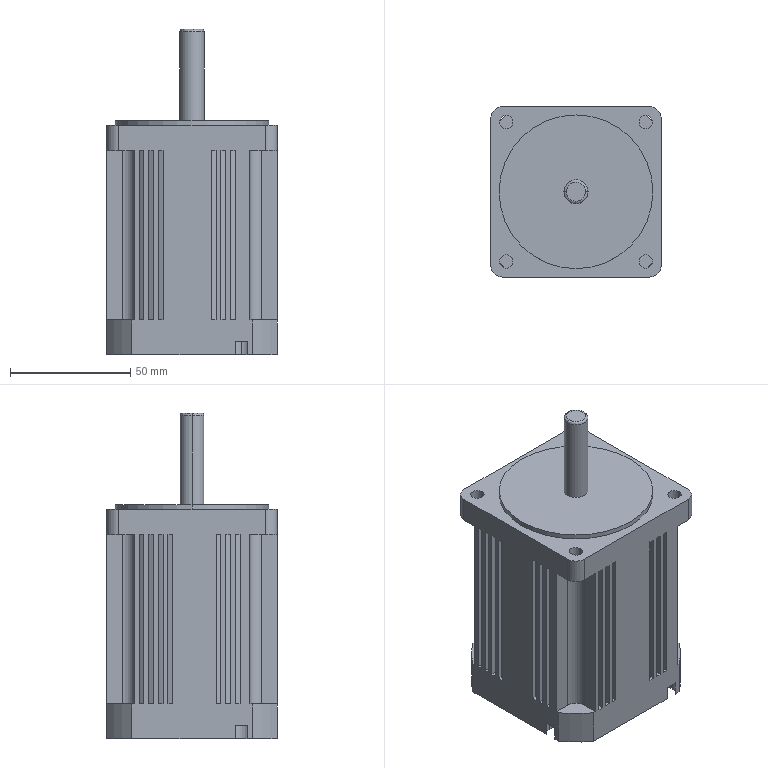Part | SolidWorks | features BaseBody 1 | 1 solid | 238 faces | box 71 x 71 x 135.5 mm | volume 435514 mm3 | plane 136 | cylinder 76 | cone 24 | spline 2 | commonest cylinder face diameters 71 x27 10 x10 8.5 x9 3.3 x8 5.3 x8 5.5 x8